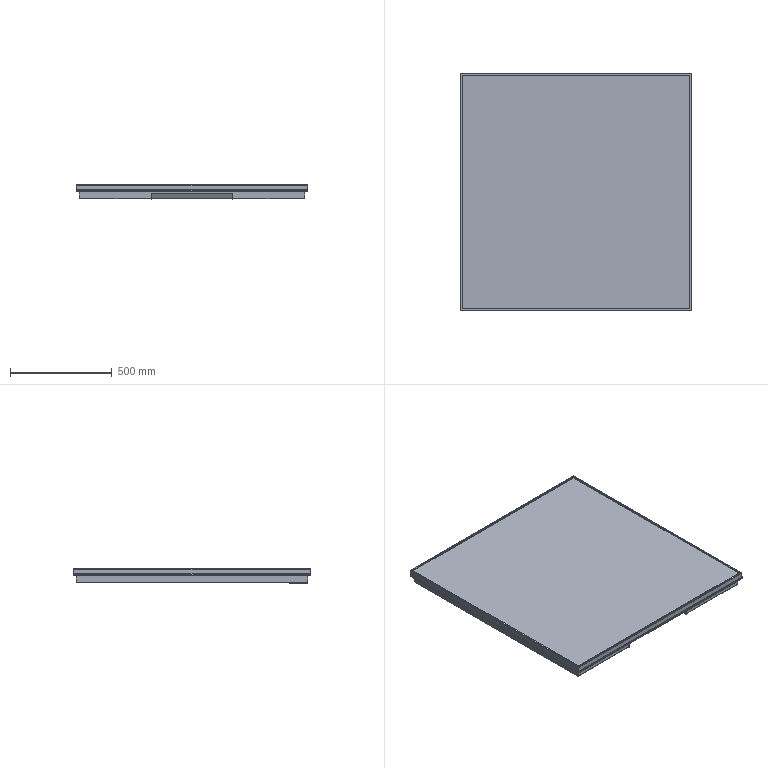Part | 7 solids | 264 faces | box 1140 x 1170 x 74.595 mm | volume 6064887 mm3 | plane 176 | cylinder 76 | spline 12 | commonest cylinder face diameters 7 x30 11 x16 0.4 x9 2.4 x9 2 x6 1 x4